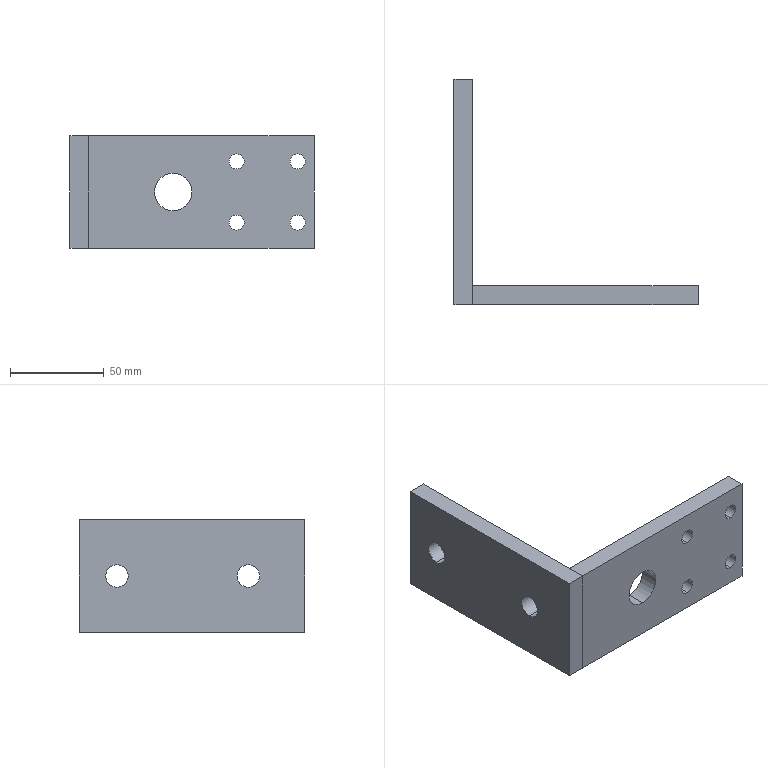Part | STEP file | BCC3 H17_1 | 2 solids | 26 faces | box 130 x 120 x 60 mm | volume 136586 mm3 | cylinder 14 | plane 12 | commonest cylinder face diameters 8 x8 12 x4 20 x2